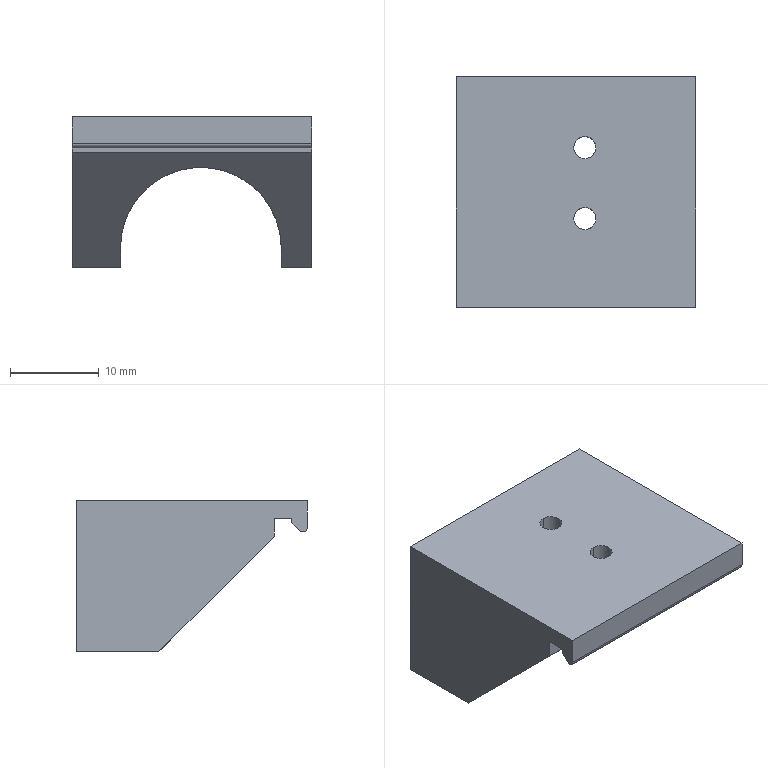NC program | NX | posted with a generic post | part box 27 x 26 x 17 mm
Lines 1769 to 2083 of 22937:
(CAVITY_MILL_COPY_COPY , TOOL : D2)
N3506 T02 M6
N3508 G54
N3510 G17 G0 G90 X-2.299 Y14.425 S9974 M3
N3512 G43 Z30. H2
N3514 Z-9.313
N3516 G94 G1 Z-10.813 F1000.
N3518 X-1.87 Y13.684
N3520 G3 X-1.003 Y13.186 R1.
N3522 G1 X-1. Y11.786
N3524 X-1.107 Y11.788
N3526 Y-5.876
N3528 G2 X-0.893 Y-5.875 R2.96
N3530 G1 Y11.788
N3532 X-1. Y11.786
N3534 X-1.003 Y13.186
N3536 G2 X-2.151 Y13.686 R1.56
N3538 G3 X-2.787 Y13.768 R0.5
N3540 G2 X-2.476 Y13.193 R1.1
N3542 G1 X-2.432 Y12.969
N3544 X-2.507 Y12.932
N3546 Y-7.178
N3548 G2 X-2.838 Y-7.925 R1.077
N3550 G3 X-2.186 Y-7.827 R0.5
N3552 G2 X0.183 Y-7.809 R1.56
N3554 G3 X0.821 Y-7.908 R0.5
N3556 G2 X0.507 Y-7.177 R1.077
N3558 G1 Y12.932
N3560 X0.431 Y12.968
N3562 X0.634 Y13.596
N3564 G2 X0.888 Y13.828 R1.465
N3566 G3 X0.196 Y13.752 R0.5
N3568 G2 X-1.003 Y13.186 R1.56
N3570 X-1.87 Y13.684 R1.
N3572 G1 X-2.299 Y14.425
N3574 Z-9.313
N3576 G0 X0.021 Y14.768 Z-9.512
N3578 G1 Z-11.012
N3580 X-0.143 Y14.489
N3582 G2 X-1.014 Y13.996 R1.
N3584 X-1.67 Y14.148 R1.56
N3586 G3 X-2.303 Y13.97 R0.5
N3588 G2 X-1.749 Y13.555 R1.551
N3590 G1 X-1.624 Y12.945
N3592 X-1.676 Y12.932
N3594 Y-7.379
N3596 G2 X-2.356 Y-8.342 R1.1
N3598 G3 X-1.727 Y-8.5 R0.5
N3600 G2 X-0.352 Y-8.498 R1.56
N3602 G1 X-0.205 Y-8.57
N3604 G3 X0.446 Y-8.375 R0.5
N3606 G2 X-0.324 Y-7.379 R1.1
N3608 G1 Y12.932
N3610 X-0.376 Y12.945
N3612 G2 X-0.064 Y13.761 R0.897
N3614 X0.269 Y13.957 R1.682
N3616 G3 X-0.355 Y14.136 R0.5
N3618 G2 X-1.014 Y13.996 R1.56
N3620 X-1.875 Y14.504 R1.
N3622 G1 X-2.035 Y14.786
N3624 Z-9.512
N3626 G0 Z30.
N3628 X-15.349 Y-9.89
N3630 Z-11.907
N3632 G1 Z-13.407
N3634 X-14.874 Y-10.505
N3636 G2 X-14.74 Y-11.496 R1.
N3638 G1 X-14.76 Y-11.544
N3640 G3 X-14.53 Y-12.176 R0.5
N3642 G2 X-13.5 Y-11.312 R1.194
N3644 G1 X13.396
N3646 G2 X14.536 Y-12.168 R1.188
N3648 G3 X14.762 Y-11.54 R0.5
N3650 G1 X14.721 Y-11.44
N3652 G2 X14.725 Y-10.254 R1.56
N3654 G3 X14.535 Y-9.642 R0.5
N3656 G2 X13.5 Y-10.37 R1.1
N3658 G1 X-13.5
N3660 G2 X-14.535 Y-9.644 R1.1
N3662 G3 X-14.724 Y-10.256 R0.5
N3664 G2 X-14.72 Y-11.449 R1.56
N3666 G1 X-14.74 Y-11.496
N3668 G2 X-15.346 Y-12.064 R1.
N3670 G1 Z-11.907
N3672 G0 X-15.301 Y-10.871 Z-12.107
N3674 G1 Z-13.607
N3676 G2 X-14.782 Y-11.508 R1.
N3678 G3 X-14.55 Y-11.811 R0.5
N3680 G2 X-13.5 Y-11.022 R1.122
N3682 G1 X13.5
N3684 G2 X14.551 Y-11.815 R1.122
N3686 G3 X14.774 Y-11.217 R0.5
N3688 G2 X14.777 Y-10.186 R1.56
N3690 G3 X14.554 Y-9.586 R0.5
N3692 G2 X13.5 Y-10.37 R1.1
N3694 G1 X-13.5
N3696 G2 X-14.554 Y-9.586 R1.1
N3698 G3 X-14.776 Y-10.187 R0.5
N3700 G2 X-14.772 Y-11.216 R1.56
N3702 G3 X-14.782 Y-11.508 R0.5
N3704 G2 X-15.041 Y-12.473 R1.
N3706 G1 X-15.2 Y-12.632
N3708 Z-12.107
N3710 G0 X-15.416 Y-11.046 Z-12.306
N3712 G1 Z-13.806
N3714 G2 X-14.746 Y-11.484 R1.
N3716 G3 X-14.562 Y-11.653 R0.5
N3718 G2 X-13.5 Y-10.822 R1.121
N3720 G1 X13.5
N3722 G2 X14.562 Y-11.66 R1.128
N3724 G3 X14.808 Y-11.069 R0.5
N3726 G2 X14.809 Y-10.14 R1.56
N3728 G3 X14.564 Y-9.548 R0.5
N3730 G2 X13.5 Y-10.37 R1.1
N3732 G1 X-13.5
N3734 G2 X-14.564 Y-9.548 R1.1
N3736 G3 X-14.809 Y-10.14 R0.5
N3738 G2 X-14.806 Y-11.064 R1.56
N3740 G3 X-14.746 Y-11.484 R0.5
N3742 G2 X-14.719 Y-11.984 R0.5
N3744 G1 X-15.2 Y-12.936
N3746 Z-12.306
N3748 G0 X-15.444 Y-11.165 Z-12.506
N3750 G1 Z-14.006
N3752 G2 X-14.683 Y-11.413 R1.
N3754 G1 X-14.571 Y-11.488
N3756 G2 X-13.5 Y-10.623 R1.121
N3758 G1 X13.5
N3760 G2 X14.57 Y-11.483 R1.121
N3762 G3 X14.832 Y-10.908 R0.5
N3764 G2 X14.837 Y-10.095 R1.56
N3766 G3 X14.573 Y-9.512 R0.5
N3768 G2 X13.5 Y-10.37 R1.1
N3770 G1 X-13.5
N3772 G2 X-14.573 Y-9.511 R1.1
N3774 G3 X-14.838 Y-10.094 R0.5
N3776 G2 X-14.834 Y-10.91 R1.56
N3778 G3 X-14.683 Y-11.413 R0.5
N3780 G2 X-14.551 Y-11.19 R0.5
N3782 G1 X-15.227 Y-11.704
N3784 Z-12.506
N3786 G0 X-15.421 Y-11.228 Z-12.706
N3788 G1 Z-14.206
N3790 G2 X-14.626 Y-11.312 R1.
N3792 G1 X-14.58 Y-11.335
N3794 G2 X-13.5 Y-10.423 R1.126
N3796 G1 X13.5
N3798 G2 X14.579 Y-11.335 R1.129
N3800 G3 X14.864 Y-10.764 R0.5
N3802 G2 X14.866 Y-10.047 R1.56
N3804 G3 X14.581 Y-9.473 R0.5
N3806 G2 X13.5 Y-10.37 R1.1
N3808 G1 X-13.5
N3810 G2 X-14.581 Y-9.472 R1.1
N3812 G3 X-14.866 Y-10.046 R0.5
N3814 G2 X-14.865 Y-10.763 R1.56
N3816 G3 X-14.626 Y-11.312 R0.5
N3818 G2 X-14.504 Y-11.084 R0.5
N3820 G1 X-15.2 Y-11.609
N3822 Z-12.706
N3824 G0 Y-11.937 Z-12.905
N3826 G1 Z-14.405
N3828 G3 X-14.585 Y-11.169 R1.
N3830 G2 X-13.893 Y-10.297 R1.138
N3832 X-14.587 Y-9.436 R1.1
N3834 G3 X-15.2 Y-8.66 R1.
N3836 G1 Z-12.905
N3838 G0 Y-11.906 Z-13.105
N3840 G1 Z-14.605
N3842 G3 X-14.59 Y-11.119 R1.
N3844 G2 X-13.958 Y-10.27 R1.1
N3846 X-14.59 Y-9.421 R1.1
N3848 G3 X-15.2 Y-8.634 R1.
N3850 G1 Z-13.105
N3852 G0 Y-11.906 Z-13.304
N3854 G1 Z-14.804
N3856 G3 X-14.59 Y-11.119 R1.
N3858 G2 X-13.958 Y-10.27 R1.1
N3860 X-14.59 Y-9.421 R1.1
N3862 G3 X-15.2 Y-8.634 R1.
N3864 G1 Z-13.304
N3866 G0 Z30.
N3868 X15.2 Y-8.661
N3870 Z-12.905
N3872 G1 Z-14.405
N3874 G3 X14.587 Y-9.436 R1.
N3876 G2 X13.893 Y-10.297 R1.1
N3878 X14.585 Y-11.175 R1.151
N3880 G3 X15.2 Y-11.943 R1.
N3882 G1 Z-12.905
N3884 G0 Y-8.634 Z-13.105
N3886 G1 Z-14.605
N3888 G3 X14.59 Y-9.421 R1.
N3890 G2 X13.958 Y-10.27 R1.1
N3892 X14.59 Y-11.119 R1.1
N3894 G3 X15.2 Y-11.906 R1.
N3896 G1 Z-13.105
N3898 G0 Y-8.634 Z-13.304
N3900 G1 Z-14.804
N3902 G3 X14.59 Y-9.421 R1.
N3904 G2 X13.958 Y-10.27 R1.1
N3906 X14.59 Y-11.119 R1.1
N3908 G3 X15.2 Y-11.906 R1.
N3910 G1 Z-13.304
N3912 G0 Z30.
(PLANAR_PROFILE , TOOL : D2)
N3914 X17.5 Y-10.27 S9500
N3916 Z-9.65
N3918 G1 Z-12.65 F1250.
N3920 X13.5
N3922 X-13.5
N3924 X-17.5
N3926 Z-9.65
N3928 G0 Z-9.8
N3930 G1 Z-12.8
N3932 X-13.5
N3934 X13.5
N3936 X17.5
N3938 Z-9.8
N3940 G0 Z-9.95
N3942 G1 Z-12.95
N3944 X13.5
N3946 X-13.5
N3948 X-17.5
N3950 Z-9.95
N3952 G0 Z-10.1
N3954 G1 Z-13.1
N3956 X-13.5
N3958 X13.5
N3960 X17.5
N3962 Z-10.1
N3964 G0 Z-10.25
N3966 G1 Z-13.25
N3968 X13.5
N3970 X-13.5
N3972 X-17.5
N3974 Z-10.25
N3976 G0 Z-10.4
N3978 G1 Z-13.4
N3980 X-13.5
N3982 X13.5
N3984 X17.5
N3986 Z-10.4
N3988 G0 Z-10.55
N3990 G1 Z-13.55
N3992 X13.5
N3994 X-13.5
N3996 X-17.5
N3998 Z-10.55
N4000 G0 Z-10.7
N4002 G1 Z-13.7
N4004 X-13.5
N4006 X13.5
N4008 X17.5
N4010 Z-10.7
N4012 G0 Z-10.85
N4014 G1 Z-13.85
N4016 X13.5
N4018 X-13.5
N4020 X-17.5
N4022 Z-10.85
N4024 G0 Z-11.
N4026 G1 Z-14.
N4028 X-13.5
N4030 X13.5
N4032 X17.5
N4034 Z-11.
N4036 G0 Z-11.15
N4038 G1 Z-14.15
N4040 X13.5
N4042 X-13.5
N4044 X-17.5
N4046 Z-11.15
N4048 G0 Z-11.3
N4050 G1 Z-14.3
N4052 X-13.5
N4054 X13.5
N4056 X17.5
N4058 Z-11.3
N4060 G0 Z-11.45
N4062 G1 Z-14.45
N4064 X13.5
N4066 X-13.5
N4068 X-17.5
N4070 Z-11.45
N4072 G0 Z-11.6
N4074 G1 Z-14.6
N4076 X-13.5
N4078 X13.5
N4080 X17.5
N4082 Z-11.6
N4084 G0 Z-11.75
N4086 G1 Z-14.75
N4088 X13.5
N4090 X-13.5
N4092 X-17.5
N4094 Z-11.75
N4096 G0 Z-11.9
N4098 G1 Z-14.9
N4100 X-13.5
N4102 X13.5
N4104 X17.5
N4106 Z-11.9
N4108 G0 Z-12.
N4110 G1 Z-15.
N4112 X13.5
N4114 X-13.5
N4116 X-17.5
N4118 Z-12.
N4120 G0 Z30.
N4122 M5